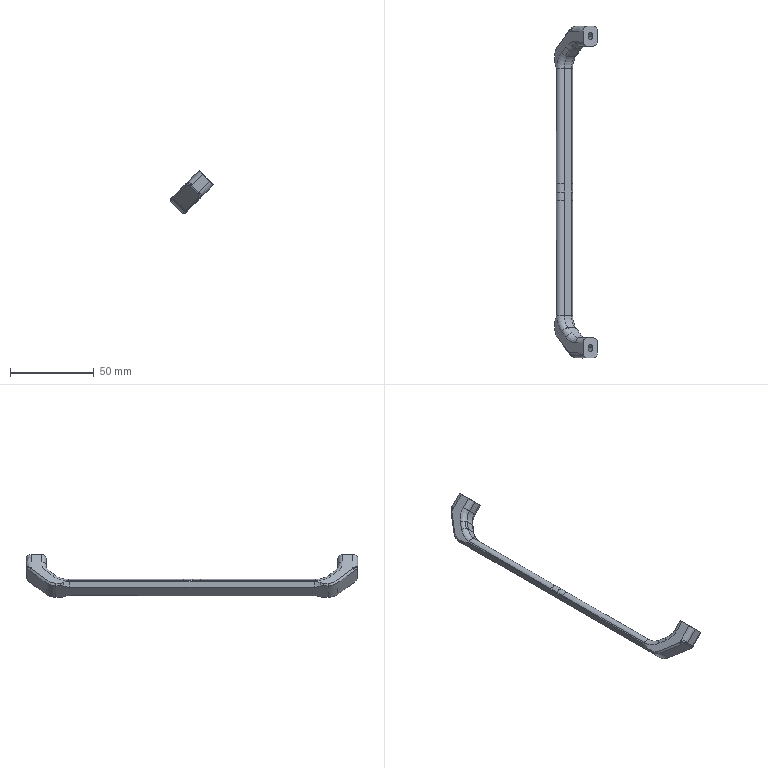Part | SolidWorks | features BaseBody 1 | 1 solid | 106 faces | box 25.601 x 198.802 x 25.601 mm | volume 16219 mm3 | cylinder 40 | spline 28 | plane 26 | cone 8 | torus 4 | commonest cylinder face diameters 6 x22 20 x6 4.2 x4 10 x4 5.998 x2 16 x2